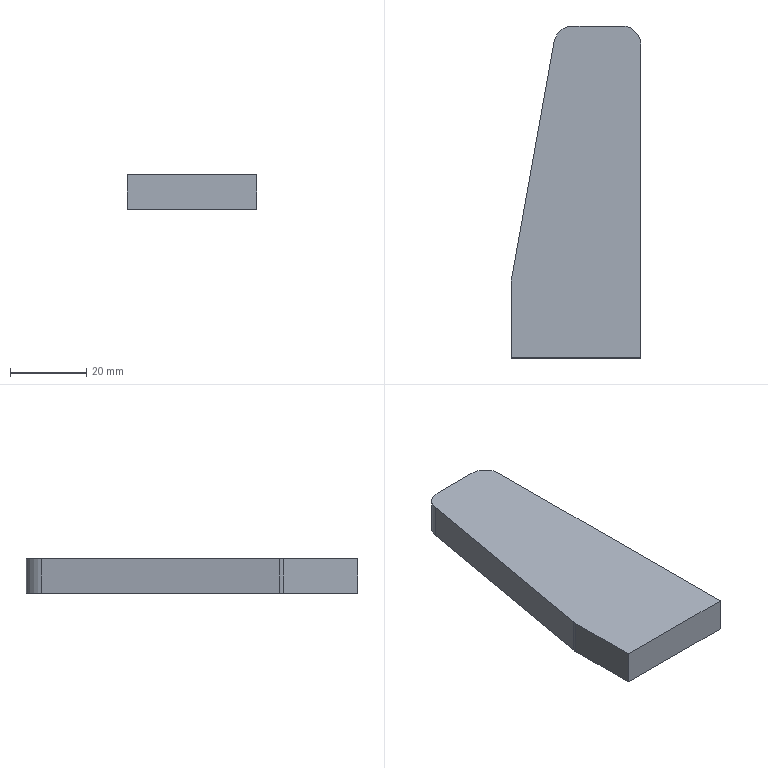Part | SolidWorks | features Extrusion 1 | 1 solid | 10 faces | box 34 x 87 x 9 mm | volume 22924 mm3 | plane 7 | cylinder 3 | commonest cylinder face diameters 10 x3
STEP:
#1=CARTESIAN_POINT('',(0.,0.,0.));
#2=VERTEX_POINT('',#1);
#3=CARTESIAN_POINT('',(0.,82.,0.));
#4=VERTEX_POINT('',#3);
#5=CARTESIAN_POINT('',(0.,0.,0.));
#6=DIRECTION('',(0.,1.,0.));
#7=VECTOR('',#6,1000.);
#8=LINE('',#5,#7);
#9=EDGE_CURVE('',#2,#4,#8,.T.);
#10=ORIENTED_EDGE('',*,*,#9,.T.);
#11=CARTESIAN_POINT('',(0.,82.,9.));
#12=VERTEX_POINT('',#11);
#13=CARTESIAN_POINT('',(0.,82.,9.));
#14=DIRECTION('',(0.,0.,-1.));
#15=VECTOR('',#14,1000.);
#16=LINE('',#13,#15);
#17=EDGE_CURVE('',#12,#4,#16,.T.);
#18=ORIENTED_EDGE('',*,*,#17,.F.);
#19=CARTESIAN_POINT('',(0.,0.,9.));
#20=VERTEX_POINT('',#19);
#21=CARTESIAN_POINT('',(0.,0.,9.));
#22=DIRECTION('',(0.,1.,0.));
#23=VECTOR('',#22,1000.);
#24=LINE('',#21,#23);
#25=EDGE_CURVE('',#20,#12,#24,.T.);
#26=ORIENTED_EDGE('',*,*,#25,.F.);
#27=CARTESIAN_POINT('',(0.,0.,9.));
#28=DIRECTION('',(0.,0.,-1.));
#29=VECTOR('',#28,1000.);
#30=LINE('',#27,#29);
#31=EDGE_CURVE('',#20,#2,#30,.T.);
#32=ORIENTED_EDGE('',*,*,#31,.T.);
#33=EDGE_LOOP('',(#10,#18,#26,#32));
#34=FACE_OUTER_BOUND('',#33,.T.);
#35=CARTESIAN_POINT('',(0.,0.,9.));
#36=DIRECTION('',(-1.,0.,0.));
#37=DIRECTION('',(0.,0.,1.));
#38=AXIS2_PLACEMENT_3D('',#35,#36,#37);
#39=PLANE('',#38);
#40=ADVANCED_FACE('',(#34),#39,.F.);
#41=CARTESIAN_POINT('',(-5.,87.,0.));
#42=VERTEX_POINT('',#41);
#43=CARTESIAN_POINT('',(-5.,82.,0.));
#44=DIRECTION('',(0.,0.,1.));
#45=DIRECTION('',(1.,0.,0.));
#46=AXIS2_PLACEMENT_3D('',#43,#44,#45);
#47=CIRCLE('',#46,5.);
#48=EDGE_CURVE('',#4,#42,#47,.T.);
#49=ORIENTED_EDGE('',*,*,#48,.T.);
#50=CARTESIAN_POINT('',(-5.,87.,9.));
#51=VERTEX_POINT('',#50);
#52=CARTESIAN_POINT('',(-5.,87.,9.));
#53=DIRECTION('',(0.,0.,-1.));
#54=VECTOR('',#53,1000.);
#55=LINE('',#52,#54);
#56=EDGE_CURVE('',#51,#42,#55,.T.);
#57=ORIENTED_EDGE('',*,*,#56,.F.);
#58=CARTESIAN_POINT('',(-5.,82.,9.));
#59=DIRECTION('',(0.,0.,1.));
#60=DIRECTION('',(1.,0.,0.));
#61=AXIS2_PLACEMENT_3D('',#58,#59,#60);
#62=CIRCLE('',#61,5.);
#63=EDGE_CURVE('',#12,#51,#62,.T.);
#64=ORIENTED_EDGE('',*,*,#63,.F.);
#65=ORIENTED_EDGE('',*,*,#17,.T.);
#66=EDGE_LOOP('',(#49,#57,#64,#65));
#67=FACE_OUTER_BOUND('',#66,.T.);
#68=CARTESIAN_POINT('',(-5.,82.,9.));
#69=DIRECTION('',(0.,0.,-1.));
#70=DIRECTION('',(-1.,0.,0.));
#71=AXIS2_PLACEMENT_3D('',#68,#69,#70);
#72=CYLINDRICAL_SURFACE('',#71,5.);
#73=ADVANCED_FACE('',(#67),#72,.T.);
#74=CARTESIAN_POINT('',(-17.816,87.,0.));
#75=VERTEX_POINT('',#74);
#76=CARTESIAN_POINT('',(-5.,87.,0.));
#77=DIRECTION('',(-1.,0.,0.));
#78=VECTOR('',#77,1000.);
#79=LINE('',#76,#78);
#80=EDGE_CURVE('',#42,#75,#79,.T.);
#81=ORIENTED_EDGE('',*,*,#80,.T.);
#82=CARTESIAN_POINT('',(-17.816,87.,9.));
#83=VERTEX_POINT('',#82);
#84=CARTESIAN_POINT('',(-17.816,87.,9.));
#85=DIRECTION('',(0.,0.,-1.));
#86=VECTOR('',#85,1000.);
#87=LINE('',#84,#86);
#88=EDGE_CURVE('',#83,#75,#87,.T.);
#89=ORIENTED_EDGE('',*,*,#88,.F.);
#90=CARTESIAN_POINT('',(-5.,87.,9.));
#91=DIRECTION('',(-1.,0.,0.));
#92=VECTOR('',#91,1000.);
#93=LINE('',#90,#92);
#94=EDGE_CURVE('',#51,#83,#93,.T.);
#95=ORIENTED_EDGE('',*,*,#94,.F.);
#96=ORIENTED_EDGE('',*,*,#56,.T.);
#97=EDGE_LOOP('',(#81,#89,#95,#96));
#98=FACE_OUTER_BOUND('',#97,.T.);
#99=CARTESIAN_POINT('',(-5.,87.,9.));
#100=DIRECTION('',(0.,-1.,0.));
#101=DIRECTION('',(0.,0.,-1.));
#102=AXIS2_PLACEMENT_3D('',#99,#100,#101);
#103=PLANE('',#102);
#104=ADVANCED_FACE('',(#98),#103,.F.);
#105=CARTESIAN_POINT('',(-22.738,82.881,0.));
#106=VERTEX_POINT('',#105);
#107=CARTESIAN_POINT('',(-17.816,82.,0.));
#108=DIRECTION('',(0.,0.,1.));
#109=DIRECTION('',(1.,0.,0.));
#110=AXIS2_PLACEMENT_3D('',#107,#108,#109);
#111=CIRCLE('',#110,5.);
#112=EDGE_CURVE('',#75,#106,#111,.T.);
#113=ORIENTED_EDGE('',*,*,#112,.T.);
#114=CARTESIAN_POINT('',(-22.738,82.881,9.));
#115=VERTEX_POINT('',#114);
#116=CARTESIAN_POINT('',(-22.738,82.881,9.));
#117=DIRECTION('',(0.,0.,-1.));
#118=VECTOR('',#117,1000.);
#119=LINE('',#116,#118);
#120=EDGE_CURVE('',#115,#106,#119,.T.);
#121=ORIENTED_EDGE('',*,*,#120,.F.);
#122=CARTESIAN_POINT('',(-17.816,82.,9.));
#123=DIRECTION('',(0.,0.,1.));
#124=DIRECTION('',(1.,0.,0.));
#125=AXIS2_PLACEMENT_3D('',#122,#123,#124);
#126=CIRCLE('',#125,5.);
#127=EDGE_CURVE('',#83,#115,#126,.T.);
#128=ORIENTED_EDGE('',*,*,#127,.F.);
#129=ORIENTED_EDGE('',*,*,#88,.T.);
#130=EDGE_LOOP('',(#113,#121,#128,#129));
#131=FACE_OUTER_BOUND('',#130,.T.);
#132=CARTESIAN_POINT('',(-17.816,82.,9.));
#133=DIRECTION('',(0.,0.,-1.));
#134=DIRECTION('',(-1.,0.,0.));
#135=AXIS2_PLACEMENT_3D('',#132,#133,#134);
#136=CYLINDRICAL_SURFACE('',#135,5.);
#137=ADVANCED_FACE('',(#131),#136,.T.);
#138=CARTESIAN_POINT('',(-33.922,20.437,0.));
#139=VERTEX_POINT('',#138);
#140=CARTESIAN_POINT('',(-33.922,20.437,0.));
#141=DIRECTION('',(-0.1763,-0.9843,0.));
#142=VECTOR('',#141,1000.);
#143=LINE('',#140,#142);
#144=EDGE_CURVE('',#106,#139,#143,.T.);
#145=ORIENTED_EDGE('',*,*,#144,.T.);
#146=CARTESIAN_POINT('',(-33.922,20.437,9.));
#147=VERTEX_POINT('',#146);
#148=CARTESIAN_POINT('',(-33.922,20.437,9.));
#149=DIRECTION('',(0.,0.,-1.));
#150=VECTOR('',#149,1000.);
#151=LINE('',#148,#150);
#152=EDGE_CURVE('',#147,#139,#151,.T.);
#153=ORIENTED_EDGE('',*,*,#152,.F.);
#154=CARTESIAN_POINT('',(-33.922,20.437,9.));
#155=DIRECTION('',(-0.1763,-0.9843,0.));
#156=VECTOR('',#155,1000.);
#157=LINE('',#154,#156);
#158=EDGE_CURVE('',#115,#147,#157,.T.);
#159=ORIENTED_EDGE('',*,*,#158,.F.);
#160=ORIENTED_EDGE('',*,*,#120,.T.);
#161=EDGE_LOOP('',(#145,#153,#159,#160));
#162=FACE_OUTER_BOUND('',#161,.T.);
#163=CARTESIAN_POINT('',(-33.922,20.437,9.));
#164=DIRECTION('',(0.9843,-0.1763,0.));
#165=DIRECTION('',(0.1763,0.9843,0.));
#166=AXIS2_PLACEMENT_3D('',#163,#164,#165);
#167=PLANE('',#166);
#168=ADVANCED_FACE('',(#162),#167,.F.);
#169=CARTESIAN_POINT('',(-34.,19.556,0.));
#170=VERTEX_POINT('',#169);
#171=CARTESIAN_POINT('',(-29.,19.556,0.));
#172=DIRECTION('',(0.,0.,1.));
#173=DIRECTION('',(-1.,0.,0.));
#174=AXIS2_PLACEMENT_3D('',#171,#172,#173);
#175=CIRCLE('',#174,5.);
#176=EDGE_CURVE('',#139,#170,#175,.T.);
#177=ORIENTED_EDGE('',*,*,#176,.T.);
#178=CARTESIAN_POINT('',(-34.,19.556,9.));
#179=VERTEX_POINT('',#178);
#180=CARTESIAN_POINT('',(-34.,19.556,9.));
#181=DIRECTION('',(0.,0.,-1.));
#182=VECTOR('',#181,1000.);
#183=LINE('',#180,#182);
#184=EDGE_CURVE('',#179,#170,#183,.T.);
#185=ORIENTED_EDGE('',*,*,#184,.F.);
#186=CARTESIAN_POINT('',(-29.,19.556,9.));
#187=DIRECTION('',(0.,0.,1.));
#188=DIRECTION('',(-1.,0.,0.));
#189=AXIS2_PLACEMENT_3D('',#186,#187,#188);
#190=CIRCLE('',#189,5.);
#191=EDGE_CURVE('',#147,#179,#190,.T.);
#192=ORIENTED_EDGE('',*,*,#191,.F.);
#193=ORIENTED_EDGE('',*,*,#152,.T.);
#194=EDGE_LOOP('',(#177,#185,#192,#193));
#195=FACE_OUTER_BOUND('',#194,.T.);
#196=CARTESIAN_POINT('',(-29.,19.556,9.));
#197=DIRECTION('',(0.,0.,-1.));
#198=DIRECTION('',(-1.,0.,0.));
#199=AXIS2_PLACEMENT_3D('',#196,#197,#198);
#200=CYLINDRICAL_SURFACE('',#199,5.);
#201=ADVANCED_FACE('',(#195),#200,.T.);
#202=CARTESIAN_POINT('',(-34.,0.,0.));
#203=VERTEX_POINT('',#202);
#204=CARTESIAN_POINT('',(-34.,0.,0.));
#205=DIRECTION('',(0.,-1.,0.));
#206=VECTOR('',#205,1000.);
#207=LINE('',#204,#206);
#208=EDGE_CURVE('',#170,#203,#207,.T.);
#209=ORIENTED_EDGE('',*,*,#208,.T.);
#210=CARTESIAN_POINT('',(-34.,0.,9.));
#211=VERTEX_POINT('',#210);
#212=CARTESIAN_POINT('',(-34.,0.,9.));
#213=DIRECTION('',(0.,0.,-1.));
#214=VECTOR('',#213,1000.);
#215=LINE('',#212,#214);
#216=EDGE_CURVE('',#211,#203,#215,.T.);
#217=ORIENTED_EDGE('',*,*,#216,.F.);
#218=CARTESIAN_POINT('',(-34.,0.,9.));
#219=DIRECTION('',(0.,-1.,0.));
#220=VECTOR('',#219,1000.);
#221=LINE('',#218,#220);
#222=EDGE_CURVE('',#179,#211,#221,.T.);
#223=ORIENTED_EDGE('',*,*,#222,.F.);
#224=ORIENTED_EDGE('',*,*,#184,.T.);
#225=EDGE_LOOP('',(#209,#217,#223,#224));
#226=FACE_OUTER_BOUND('',#225,.T.);
#227=CARTESIAN_POINT('',(-34.,0.,9.));
#228=DIRECTION('',(1.,0.,0.));
#229=DIRECTION('',(0.,0.,-1.));
#230=AXIS2_PLACEMENT_3D('',#227,#228,#229);
#231=PLANE('',#230);
#232=ADVANCED_FACE('',(#226),#231,.F.);
#233=CARTESIAN_POINT('',(0.,0.,0.));
#234=DIRECTION('',(1.,0.,0.));
#235=VECTOR('',#234,1000.);
#236=LINE('',#233,#235);
#237=EDGE_CURVE('',#203,#2,#236,.T.);
#238=ORIENTED_EDGE('',*,*,#237,.T.);
#239=ORIENTED_EDGE('',*,*,#31,.F.);
#240=CARTESIAN_POINT('',(0.,0.,9.));
#241=DIRECTION('',(1.,0.,0.));
#242=VECTOR('',#241,1000.);
#243=LINE('',#240,#242);
#244=EDGE_CURVE('',#211,#20,#243,.T.);
#245=ORIENTED_EDGE('',*,*,#244,.F.);
#246=ORIENTED_EDGE('',*,*,#216,.T.);
#247=EDGE_LOOP('',(#238,#239,#245,#246));
#248=FACE_OUTER_BOUND('',#247,.T.);
#249=CARTESIAN_POINT('',(0.,0.,9.));
#250=DIRECTION('',(0.,1.,0.));
#251=DIRECTION('',(-1.,0.,0.));
#252=AXIS2_PLACEMENT_3D('',#249,#250,#251);
#253=PLANE('',#252);
#254=ADVANCED_FACE('',(#248),#253,.F.);
#255=ORIENTED_EDGE('',*,*,#25,.T.);
#256=ORIENTED_EDGE('',*,*,#63,.T.);
#257=ORIENTED_EDGE('',*,*,#94,.T.);
#258=ORIENTED_EDGE('',*,*,#127,.T.);
#259=ORIENTED_EDGE('',*,*,#158,.T.);
#260=ORIENTED_EDGE('',*,*,#191,.T.);
#261=ORIENTED_EDGE('',*,*,#222,.T.);
#262=ORIENTED_EDGE('',*,*,#244,.T.);
#263=EDGE_LOOP('',(#255,#256,#257,#258,#259,#260,#261,#262));
#264=FACE_OUTER_BOUND('',#263,.T.);
#265=CARTESIAN_POINT('',(-5.,82.,9.));
#266=DIRECTION('',(0.,0.,1.));
#267=DIRECTION('',(1.,0.,0.));
#268=AXIS2_PLACEMENT_3D('',#265,#266,#267);
#269=PLANE('',#268);
#270=ADVANCED_FACE('',(#264),#269,.T.);
#271=ORIENTED_EDGE('',*,*,#9,.F.);
#272=ORIENTED_EDGE('',*,*,#237,.F.);
#273=ORIENTED_EDGE('',*,*,#208,.F.);
#274=ORIENTED_EDGE('',*,*,#176,.F.);
#275=ORIENTED_EDGE('',*,*,#144,.F.);
#276=ORIENTED_EDGE('',*,*,#112,.F.);
#277=ORIENTED_EDGE('',*,*,#80,.F.);
#278=ORIENTED_EDGE('',*,*,#48,.F.);
#279=EDGE_LOOP('',(#271,#272,#273,#274,#275,#276,#277,#278));
#280=FACE_OUTER_BOUND('',#279,.T.);
#281=CARTESIAN_POINT('',(-5.,82.,0.));
#282=DIRECTION('',(0.,0.,1.));
#283=DIRECTION('',(1.,0.,0.));
#284=AXIS2_PLACEMENT_3D('',#281,#282,#283);
#285=PLANE('',#284);
#286=ADVANCED_FACE('',(#280),#285,.F.);
#287=CLOSED_SHELL('',(#40,#73,#104,#137,#168,#201,#232,#254,#270,#286));
#288=MANIFOLD_SOLID_BREP('',#287);
#289=CARTESIAN_POINT('',(0.,0.,0.));
#290=DIRECTION('',(0.,0.,1.));
#291=DIRECTION('',(1.,0.,0.));
#292=AXIS2_PLACEMENT_3D('',#289,#290,#291);
#293=(LENGTH_UNIT()NAMED_UNIT(*)SI_UNIT(.MILLI.,.METRE.));
#294=UNCERTAINTY_MEASURE_WITH_UNIT(LENGTH_MEASURE(0.00001),#293,'','');
#295=(NAMED_UNIT(*)PLANE_ANGLE_UNIT()SI_UNIT($,.RADIAN.));
#296=(NAMED_UNIT(*)SI_UNIT($,.STERADIAN.)SOLID_ANGLE_UNIT());
#297=(GEOMETRIC_REPRESENTATION_CONTEXT(3)GLOBAL_UNCERTAINTY_ASSIGNED_CONTEXT((#294))GLOBAL_UNIT_ASSIGNED_CONTEXT((#293,#295,#296))REPRESENTATION_CONTEXT('',''));
#298=ADVANCED_BREP_SHAPE_REPRESENTATION('',(#288,#292),#297);